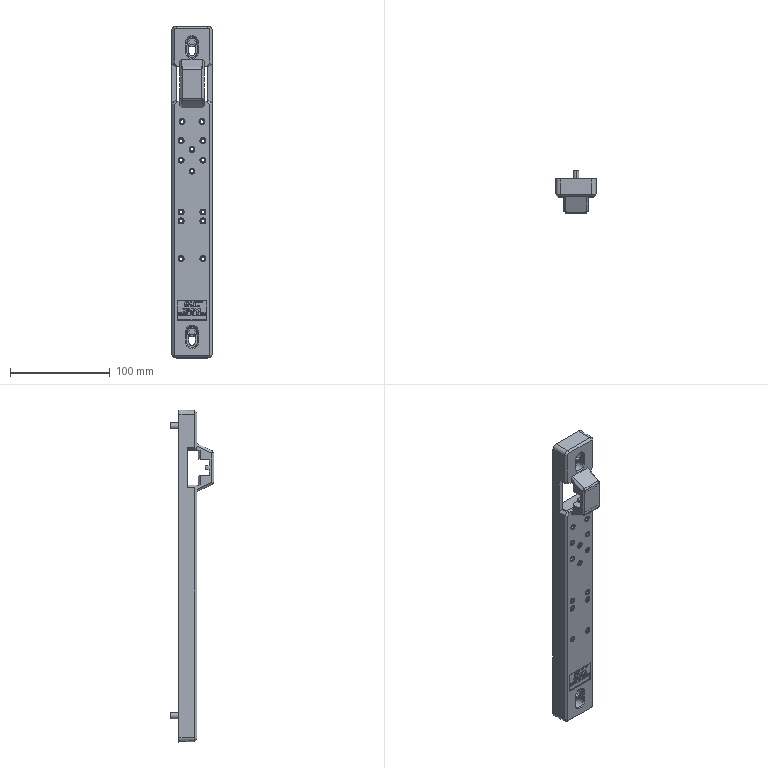Part | SolidWorks | features BaseBody 17 | 17 solids | 7024 faces | volume 135185 mm3 | plane 4749 | cylinder 1851 | spline 224 | cone 172 | torus 24 | sphere 4 | commonest cylinder face diameters 6 x1684 2 x66 5 x36 3.6 x28 4 x12 4.677 x7